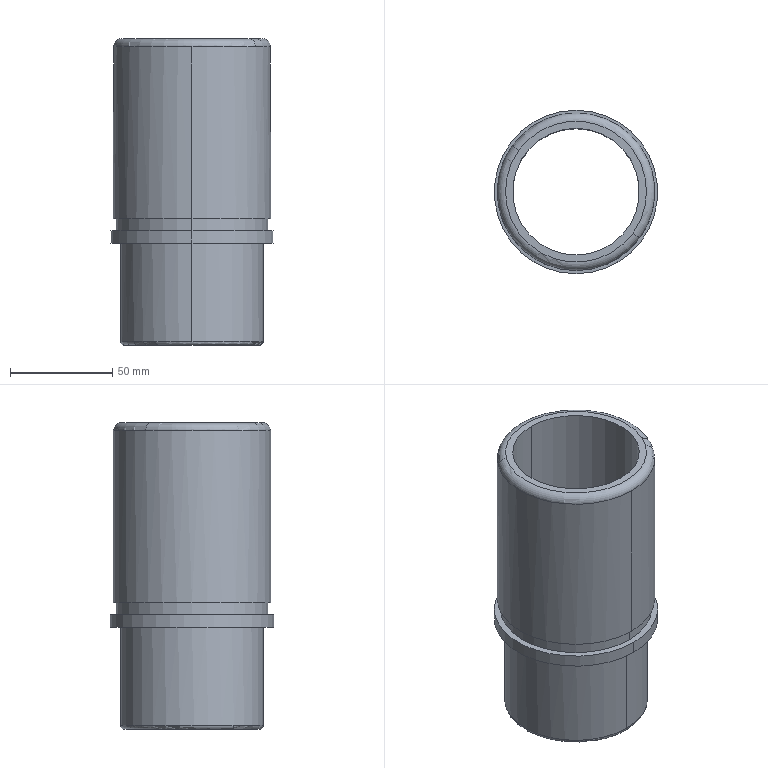Part | 1 solid | 19 faces | box 80 x 80 x 150 mm | volume 204312 mm3 | cylinder 10 | plane 5 | torus 4 | commonest cylinder face diameters 62 x2 70 x2 74.001 x2 77 x2 80 x2
STEP:
#1=CARTESIAN_POINT('',(0.,0.,0.));
#2=DIRECTION('',(0.,0.,1.));
#3=DIRECTION('',(1.,0.,0.));
#4=AXIS2_PLACEMENT_3D('',#1,#2,#3);
#5=CARTESIAN_POINT('',(-480.,16.5,-286.55));
#6=VERTEX_POINT('',#5);
#7=CARTESIAN_POINT('',(-480.,16.5,-334.55));
#8=VERTEX_POINT('',#7);
#9=CARTESIAN_POINT('',(-480.,16.5,-286.55));
#10=DIRECTION('',(0.,0.,-1.));
#11=VECTOR('',#10,1.);
#12=LINE('',#9,#11);
#13=CARTESIAN_POINT('',(-480.,-18.5,-169.951));
#14=DIRECTION('',(0.,0.,-1.));
#15=DIRECTION('',(-1.,0.,0.));
#16=AXIS2_PLACEMENT_3D('',#13,#14,#15);
#17=CYLINDRICAL_SURFACE('',#16,35.);
#18=CARTESIAN_POINT('',(1.571,116.599));
#19=DIRECTION('',(0.,1.));
#20=VECTOR('',#19,1.);
#21=LINE('',#18,#20);
#22=(GEOMETRIC_REPRESENTATION_CONTEXT(2)PARAMETRIC_REPRESENTATION_CONTEXT()REPRESENTATION_CONTEXT('',''));
#23=DEFINITIONAL_REPRESENTATION('',(#21),#22);
#24=PCURVE('',#17,#23);
#25=CARTESIAN_POINT('',(-480.,-18.5,-169.951));
#26=DIRECTION('',(0.,0.,-1.));
#27=DIRECTION('',(1.,0.,0.));
#28=AXIS2_PLACEMENT_3D('',#25,#26,#27);
#29=CYLINDRICAL_SURFACE('',#28,35.);
#30=CARTESIAN_POINT('',(4.712,116.599));
#31=DIRECTION('',(0.,1.));
#32=VECTOR('',#31,1.);
#33=LINE('',#30,#32);
#34=(GEOMETRIC_REPRESENTATION_CONTEXT(2)PARAMETRIC_REPRESENTATION_CONTEXT()REPRESENTATION_CONTEXT('',''));
#35=DEFINITIONAL_REPRESENTATION('',(#33),#34);
#36=PCURVE('',#29,#35);
#37=SURFACE_CURVE('',#12,(#24,#36),.PCURVE_S1.);
#38=EDGE_CURVE('',#6,#8,#37,.T.);
#39=ORIENTED_EDGE('',*,*,#38,.F.);
#40=CARTESIAN_POINT('',(-480.,-53.5,-286.55));
#41=VERTEX_POINT('',#40);
#42=CARTESIAN_POINT('',(-480.,-18.5,-286.55));
#43=DIRECTION('',(0.,0.,-1.));
#44=DIRECTION('',(0.,-1.,0.));
#45=AXIS2_PLACEMENT_3D('',#42,#43,#44);
#46=CIRCLE('',#45,35.);
#47=CARTESIAN_POINT('',(-1.571,116.599));
#48=DIRECTION('',(1.,0.));
#49=VECTOR('',#48,1.);
#50=LINE('',#47,#49);
#51=(GEOMETRIC_REPRESENTATION_CONTEXT(2)PARAMETRIC_REPRESENTATION_CONTEXT()REPRESENTATION_CONTEXT('',''));
#52=DEFINITIONAL_REPRESENTATION('',(#50),#51);
#53=PCURVE('',#17,#52);
#54=CARTESIAN_POINT('',(-530.585,-18.5,-286.55));
#55=DIRECTION('',(0.,0.,-1.));
#56=DIRECTION('',(0.,-1.,0.));
#57=AXIS2_PLACEMENT_3D('',#54,#55,#56);
#58=PLANE('',#57);
#59=CARTESIAN_POINT('',(0.,-50.585));
#60=DIRECTION('',(1.,0.));
#61=AXIS2_PLACEMENT_2D('',#59,#60);
#62=CIRCLE('',#61,35.);
#63=(GEOMETRIC_REPRESENTATION_CONTEXT(2)PARAMETRIC_REPRESENTATION_CONTEXT()REPRESENTATION_CONTEXT('',''));
#64=DEFINITIONAL_REPRESENTATION('',(#62),#63);
#65=PCURVE('',#58,#64);
#66=SURFACE_CURVE('',#46,(#53,#65),.PCURVE_S1.);
#67=EDGE_CURVE('',#6,#41,#66,.T.);
#68=ORIENTED_EDGE('',*,*,#67,.T.);
#69=CARTESIAN_POINT('',(-480.,-53.5,-334.55));
#70=VERTEX_POINT('',#69);
#71=CARTESIAN_POINT('',(-480.,-53.5,-286.55));
#72=DIRECTION('',(0.,0.,-1.));
#73=VECTOR('',#72,1.);
#74=LINE('',#71,#73);
#75=CARTESIAN_POINT('',(4.712,116.599));
#76=DIRECTION('',(0.,1.));
#77=VECTOR('',#76,1.);
#78=LINE('',#75,#77);
#79=(GEOMETRIC_REPRESENTATION_CONTEXT(2)PARAMETRIC_REPRESENTATION_CONTEXT()REPRESENTATION_CONTEXT('',''));
#80=DEFINITIONAL_REPRESENTATION('',(#78),#79);
#81=PCURVE('',#17,#80);
#82=CARTESIAN_POINT('',(1.571,116.599));
#83=DIRECTION('',(0.,1.));
#84=VECTOR('',#83,1.);
#85=LINE('',#82,#84);
#86=(GEOMETRIC_REPRESENTATION_CONTEXT(2)PARAMETRIC_REPRESENTATION_CONTEXT()REPRESENTATION_CONTEXT('',''));
#87=DEFINITIONAL_REPRESENTATION('',(#85),#86);
#88=PCURVE('',#29,#87);
#89=SURFACE_CURVE('',#74,(#81,#88),.PCURVE_S1.);
#90=EDGE_CURVE('',#41,#70,#89,.T.);
#91=ORIENTED_EDGE('',*,*,#90,.T.);
#92=CARTESIAN_POINT('',(-451.684,2.072,-334.55));
#93=VERTEX_POINT('',#92);
#94=CARTESIAN_POINT('',(-480.,-18.5,-334.55));
#95=DIRECTION('',(0.,0.,-1.));
#96=DIRECTION('',(0.,-1.,0.));
#97=AXIS2_PLACEMENT_3D('',#94,#95,#96);
#98=CIRCLE('',#97,35.);
#99=CARTESIAN_POINT('',(-1.571,164.599));
#100=DIRECTION('',(1.,0.));
#101=VECTOR('',#100,1.);
#102=LINE('',#99,#101);
#103=(GEOMETRIC_REPRESENTATION_CONTEXT(2)PARAMETRIC_REPRESENTATION_CONTEXT()REPRESENTATION_CONTEXT('',''));
#104=DEFINITIONAL_REPRESENTATION('',(#102),#103);
#105=PCURVE('',#17,#104);
#106=CARTESIAN_POINT('',(-480.,-18.5,-334.55));
#107=DIRECTION('',(0.,0.,-1.));
#108=DIRECTION('',(-0.5878,0.809,0.));
#109=AXIS2_PLACEMENT_3D('',#106,#107,#108);
#110=TOROIDAL_SURFACE('',#109,33.,2.);
#111=CARTESIAN_POINT('',(-2.513,0.));
#112=DIRECTION('',(1.,0.));
#113=VECTOR('',#112,1.);
#114=LINE('',#111,#113);
#115=(GEOMETRIC_REPRESENTATION_CONTEXT(2)PARAMETRIC_REPRESENTATION_CONTEXT()REPRESENTATION_CONTEXT('',''));
#116=DEFINITIONAL_REPRESENTATION('',(#114),#115);
#117=PCURVE('',#110,#116);
#118=SURFACE_CURVE('',#98,(#105,#117),.PCURVE_S1.);
#119=EDGE_CURVE('',#93,#70,#118,.T.);
#120=ORIENTED_EDGE('',*,*,#119,.F.);
#121=CARTESIAN_POINT('',(-480.,-18.5,-334.55));
#122=DIRECTION('',(0.,0.,-1.));
#123=DIRECTION('',(0.,-1.,0.));
#124=AXIS2_PLACEMENT_3D('',#121,#122,#123);
#125=CIRCLE('',#124,35.);
#126=CARTESIAN_POINT('',(-1.571,164.599));
#127=DIRECTION('',(1.,0.));
#128=VECTOR('',#127,1.);
#129=LINE('',#126,#128);
#130=(GEOMETRIC_REPRESENTATION_CONTEXT(2)PARAMETRIC_REPRESENTATION_CONTEXT()REPRESENTATION_CONTEXT('',''));
#131=DEFINITIONAL_REPRESENTATION('',(#129),#130);
#132=PCURVE('',#17,#131);
#133=CARTESIAN_POINT('',(-480.,-18.5,-334.55));
#134=DIRECTION('',(0.,0.,-1.));
#135=DIRECTION('',(0.5878,-0.809,0.));
#136=AXIS2_PLACEMENT_3D('',#133,#134,#135);
#137=TOROIDAL_SURFACE('',#136,33.,2.);
#138=CARTESIAN_POINT('',(0.6283,0.));
#139=DIRECTION('',(1.,0.));
#140=VECTOR('',#139,1.);
#141=LINE('',#138,#140);
#142=(GEOMETRIC_REPRESENTATION_CONTEXT(2)PARAMETRIC_REPRESENTATION_CONTEXT()REPRESENTATION_CONTEXT('',''));
#143=DEFINITIONAL_REPRESENTATION('',(#141),#142);
#144=PCURVE('',#137,#143);
#145=SURFACE_CURVE('',#125,(#132,#144),.PCURVE_S1.);
#146=EDGE_CURVE('',#8,#93,#145,.T.);
#147=ORIENTED_EDGE('',*,*,#146,.F.);
#148=EDGE_LOOP('',(#39,#68,#91,#120,#147));
#149=FACE_BOUND('',#148,.T.);
#150=ADVANCED_FACE('',(#149),#17,.T.);
#151=CARTESIAN_POINT('',(-480.,-58.5,-286.55));
#152=VERTEX_POINT('',#151);
#153=CARTESIAN_POINT('',(-480.,21.5,-286.55));
#154=VERTEX_POINT('',#153);
#155=CARTESIAN_POINT('',(-480.,-18.5,-286.55));
#156=DIRECTION('',(0.,0.,-1.));
#157=DIRECTION('',(0.,-1.,0.));
#158=AXIS2_PLACEMENT_3D('',#155,#156,#157);
#159=CIRCLE('',#158,40.);
#160=CARTESIAN_POINT('',(0.,-50.585));
#161=DIRECTION('',(1.,0.));
#162=AXIS2_PLACEMENT_2D('',#160,#161);
#163=CIRCLE('',#162,40.);
#164=(GEOMETRIC_REPRESENTATION_CONTEXT(2)PARAMETRIC_REPRESENTATION_CONTEXT()REPRESENTATION_CONTEXT('',''));
#165=DEFINITIONAL_REPRESENTATION('',(#163),#164);
#166=PCURVE('',#58,#165);
#167=CARTESIAN_POINT('',(-480.,-18.5,-169.951));
#168=DIRECTION('',(0.,0.,-1.));
#169=DIRECTION('',(1.,0.,0.));
#170=AXIS2_PLACEMENT_3D('',#167,#168,#169);
#171=CYLINDRICAL_SURFACE('',#170,40.);
#172=CARTESIAN_POINT('',(1.571,116.599));
#173=DIRECTION('',(1.,0.));
#174=VECTOR('',#173,1.);
#175=LINE('',#172,#174);
#176=(GEOMETRIC_REPRESENTATION_CONTEXT(2)PARAMETRIC_REPRESENTATION_CONTEXT()REPRESENTATION_CONTEXT('',''));
#177=DEFINITIONAL_REPRESENTATION('',(#175),#176);
#178=PCURVE('',#171,#177);
#179=SURFACE_CURVE('',#159,(#166,#178),.PCURVE_S1.);
#180=EDGE_CURVE('',#152,#154,#179,.T.);
#181=ORIENTED_EDGE('',*,*,#180,.T.);
#182=CARTESIAN_POINT('',(-480.,-18.5,-286.55));
#183=DIRECTION('',(0.,0.,-1.));
#184=DIRECTION('',(0.,-1.,0.));
#185=AXIS2_PLACEMENT_3D('',#182,#183,#184);
#186=CIRCLE('',#185,40.);
#187=CARTESIAN_POINT('',(0.,-50.585));
#188=DIRECTION('',(1.,0.));
#189=AXIS2_PLACEMENT_2D('',#187,#188);
#190=CIRCLE('',#189,40.);
#191=(GEOMETRIC_REPRESENTATION_CONTEXT(2)PARAMETRIC_REPRESENTATION_CONTEXT()REPRESENTATION_CONTEXT('',''));
#192=DEFINITIONAL_REPRESENTATION('',(#190),#191);
#193=PCURVE('',#58,#192);
#194=CARTESIAN_POINT('',(-480.,-18.5,-169.951));
#195=DIRECTION('',(0.,0.,-1.));
#196=DIRECTION('',(-1.,0.,0.));
#197=AXIS2_PLACEMENT_3D('',#194,#195,#196);
#198=CYLINDRICAL_SURFACE('',#197,40.);
#199=CARTESIAN_POINT('',(-1.571,116.599));
#200=DIRECTION('',(1.,0.));
#201=VECTOR('',#200,1.);
#202=LINE('',#199,#201);
#203=(GEOMETRIC_REPRESENTATION_CONTEXT(2)PARAMETRIC_REPRESENTATION_CONTEXT()REPRESENTATION_CONTEXT('',''));
#204=DEFINITIONAL_REPRESENTATION('',(#202),#203);
#205=PCURVE('',#198,#204);
#206=SURFACE_CURVE('',#186,(#193,#205),.PCURVE_S1.);
#207=EDGE_CURVE('',#154,#152,#206,.T.);
#208=ORIENTED_EDGE('',*,*,#207,.T.);
#209=EDGE_LOOP('',(#181,#208));
#210=FACE_BOUND('',#209,.T.);
#211=ORIENTED_EDGE('',*,*,#67,.F.);
#212=CARTESIAN_POINT('',(-480.,-18.5,-286.55));
#213=DIRECTION('',(0.,0.,-1.));
#214=DIRECTION('',(0.,-1.,0.));
#215=AXIS2_PLACEMENT_3D('',#212,#213,#214);
#216=CIRCLE('',#215,35.);
#217=CARTESIAN_POINT('',(0.,-50.585));
#218=DIRECTION('',(1.,0.));
#219=AXIS2_PLACEMENT_2D('',#217,#218);
#220=CIRCLE('',#219,35.);
#221=(GEOMETRIC_REPRESENTATION_CONTEXT(2)PARAMETRIC_REPRESENTATION_CONTEXT()REPRESENTATION_CONTEXT('',''));
#222=DEFINITIONAL_REPRESENTATION('',(#220),#221);
#223=PCURVE('',#58,#222);
#224=CARTESIAN_POINT('',(1.571,116.599));
#225=DIRECTION('',(1.,0.));
#226=VECTOR('',#225,1.);
#227=LINE('',#224,#226);
#228=(GEOMETRIC_REPRESENTATION_CONTEXT(2)PARAMETRIC_REPRESENTATION_CONTEXT()REPRESENTATION_CONTEXT('',''));
#229=DEFINITIONAL_REPRESENTATION('',(#227),#228);
#230=PCURVE('',#29,#229);
#231=SURFACE_CURVE('',#216,(#223,#230),.PCURVE_S1.);
#232=EDGE_CURVE('',#41,#6,#231,.T.);
#233=ORIENTED_EDGE('',*,*,#232,.F.);
#234=EDGE_LOOP('',(#211,#233));
#235=FACE_BOUND('',#234,.T.);
#236=ADVANCED_FACE('',(#210,#235),#58,.T.);
#237=CARTESIAN_POINT('',(-480.,21.5,-280.55));
#238=VERTEX_POINT('',#237);
#239=CARTESIAN_POINT('',(-480.,21.5,-280.55));
#240=DIRECTION('',(0.,0.,-1.));
#241=VECTOR('',#240,1.);
#242=LINE('',#239,#241);
#243=CARTESIAN_POINT('',(1.571,110.599));
#244=DIRECTION('',(0.,1.));
#245=VECTOR('',#244,1.);
#246=LINE('',#243,#245);
#247=(GEOMETRIC_REPRESENTATION_CONTEXT(2)PARAMETRIC_REPRESENTATION_CONTEXT()REPRESENTATION_CONTEXT('',''));
#248=DEFINITIONAL_REPRESENTATION('',(#246),#247);
#249=PCURVE('',#198,#248);
#250=CARTESIAN_POINT('',(4.712,110.599));
#251=DIRECTION('',(0.,1.));
#252=VECTOR('',#251,1.);
#253=LINE('',#250,#252);
#254=(GEOMETRIC_REPRESENTATION_CONTEXT(2)PARAMETRIC_REPRESENTATION_CONTEXT()REPRESENTATION_CONTEXT('',''));
#255=DEFINITIONAL_REPRESENTATION('',(#253),#254);
#256=PCURVE('',#171,#255);
#257=SURFACE_CURVE('',#242,(#249,#256),.PCURVE_S1.);
#258=EDGE_CURVE('',#238,#154,#257,.T.);
#259=ORIENTED_EDGE('',*,*,#258,.F.);
#260=CARTESIAN_POINT('',(-480.,-58.5,-280.55));
#261=VERTEX_POINT('',#260);
#262=CARTESIAN_POINT('',(-480.,-18.5,-280.55));
#263=DIRECTION('',(0.,0.,-1.));
#264=DIRECTION('',(0.,-1.,0.));
#265=AXIS2_PLACEMENT_3D('',#262,#263,#264);
#266=CIRCLE('',#265,40.);
#267=CARTESIAN_POINT('',(-1.571,110.599));
#268=DIRECTION('',(1.,0.));
#269=VECTOR('',#268,1.);
#270=LINE('',#267,#269);
#271=(GEOMETRIC_REPRESENTATION_CONTEXT(2)PARAMETRIC_REPRESENTATION_CONTEXT()REPRESENTATION_CONTEXT('',''));
#272=DEFINITIONAL_REPRESENTATION('',(#270),#271);
#273=PCURVE('',#198,#272);
#274=CARTESIAN_POINT('',(-539.585,-18.5,-280.55));
#275=DIRECTION('',(0.,0.,1.));
#276=DIRECTION('',(0.,1.,0.));
#277=AXIS2_PLACEMENT_3D('',#274,#275,#276);
#278=PLANE('',#277);
#279=CARTESIAN_POINT('',(-40.,-59.585));
#280=CARTESIAN_POINT('',(-40.,9.697));
#281=CARTESIAN_POINT('',(20.,-24.944));
#282=CARTESIAN_POINT('',(80.,-59.585));
#283=CARTESIAN_POINT('',(20.,-94.226));
#284=CARTESIAN_POINT('',(-40.,-128.867));
#285=CARTESIAN_POINT('',(-40.,-59.585));
#286=(BOUNDED_CURVE()B_SPLINE_CURVE(2,(#279,#280,#281,#282,#283,#284,#285),.UNSPECIFIED.,.T.,.F.)B_SPLINE_CURVE_WITH_KNOTS((1,2,2,2,2,1),(-2.094,0.,2.094,4.189,6.283,8.378),.UNSPECIFIED.)CURVE()GEOMETRIC_REPRESENTATION_ITEM()RATIONAL_B_SPLINE_CURVE((1.,0.5,1.,0.5,1.,0.5,1.))REPRESENTATION_ITEM(''));
#287=(GEOMETRIC_REPRESENTATION_CONTEXT(2)PARAMETRIC_REPRESENTATION_CONTEXT()REPRESENTATION_CONTEXT('',''));
#288=DEFINITIONAL_REPRESENTATION('',(#286),#287);
#289=PCURVE('',#278,#288);
#290=SURFACE_CURVE('',#266,(#273,#289),.PCURVE_S1.);
#291=EDGE_CURVE('',#238,#261,#290,.T.);
#292=ORIENTED_EDGE('',*,*,#291,.T.);
#293=CARTESIAN_POINT('',(-480.,-58.5,-280.55));
#294=DIRECTION('',(0.,0.,-1.));
#295=VECTOR('',#294,1.);
#296=LINE('',#293,#295);
#297=CARTESIAN_POINT('',(4.712,110.599));
#298=DIRECTION('',(0.,1.));
#299=VECTOR('',#298,1.);
#300=LINE('',#297,#299);
#301=(GEOMETRIC_REPRESENTATION_CONTEXT(2)PARAMETRIC_REPRESENTATION_CONTEXT()REPRESENTATION_CONTEXT('',''));
#302=DEFINITIONAL_REPRESENTATION('',(#300),#301);
#303=PCURVE('',#198,#302);
#304=CARTESIAN_POINT('',(1.571,110.599));
#305=DIRECTION('',(0.,1.));
#306=VECTOR('',#305,1.);
#307=LINE('',#304,#306);
#308=(GEOMETRIC_REPRESENTATION_CONTEXT(2)PARAMETRIC_REPRESENTATION_CONTEXT()REPRESENTATION_CONTEXT('',''));
#309=DEFINITIONAL_REPRESENTATION('',(#307),#308);
#310=PCURVE('',#171,#309);
#311=SURFACE_CURVE('',#296,(#303,#310),.PCURVE_S1.);
#312=EDGE_CURVE('',#261,#152,#311,.T.);
#313=ORIENTED_EDGE('',*,*,#312,.T.);
#314=ORIENTED_EDGE('',*,*,#207,.F.);
#315=EDGE_LOOP('',(#259,#292,#313,#314));
#316=FACE_BOUND('',#315,.T.);
#317=ADVANCED_FACE('',(#316),#198,.T.);
#318=ORIENTED_EDGE('',*,*,#291,.F.);
#319=CARTESIAN_POINT('',(-480.,-18.5,-280.55));
#320=DIRECTION('',(0.,0.,-1.));
#321=DIRECTION('',(0.,-1.,0.));
#322=AXIS2_PLACEMENT_3D('',#319,#320,#321);
#323=CIRCLE('',#322,40.);
#324=CARTESIAN_POINT('',(-40.,-59.585));
#325=CARTESIAN_POINT('',(-40.,9.697));
#326=CARTESIAN_POINT('',(20.,-24.944));
#327=CARTESIAN_POINT('',(80.,-59.585));
#328=CARTESIAN_POINT('',(20.,-94.226));
#329=CARTESIAN_POINT('',(-40.,-128.867));
#330=CARTESIAN_POINT('',(-40.,-59.585));
#331=(BOUNDED_CURVE()B_SPLINE_CURVE(2,(#324,#325,#326,#327,#328,#329,#330),.UNSPECIFIED.,.T.,.F.)B_SPLINE_CURVE_WITH_KNOTS((1,2,2,2,2,1),(-2.094,0.,2.094,4.189,6.283,8.378),.UNSPECIFIED.)CURVE()GEOMETRIC_REPRESENTATION_ITEM()RATIONAL_B_SPLINE_CURVE((1.,0.5,1.,0.5,1.,0.5,1.))REPRESENTATION_ITEM(''));
#332=(GEOMETRIC_REPRESENTATION_CONTEXT(2)PARAMETRIC_REPRESENTATION_CONTEXT()REPRESENTATION_CONTEXT('',''));
#333=DEFINITIONAL_REPRESENTATION('',(#331),#332);
#334=PCURVE('',#278,#333);
#335=CARTESIAN_POINT('',(1.571,110.599));
#336=DIRECTION('',(1.,0.));
#337=VECTOR('',#336,1.);
#338=LINE('',#335,#337);
#339=(GEOMETRIC_REPRESENTATION_CONTEXT(2)PARAMETRIC_REPRESENTATION_CONTEXT()REPRESENTATION_CONTEXT('',''));
#340=DEFINITIONAL_REPRESENTATION('',(#338),#339);
#341=PCURVE('',#171,#340);
#342=SURFACE_CURVE('',#323,(#334,#341),.PCURVE_S1.);
#343=EDGE_CURVE('',#261,#238,#342,.T.);
#344=ORIENTED_EDGE('',*,*,#343,.F.);
#345=EDGE_LOOP('',(#318,#344));
#346=FACE_BOUND('',#345,.T.);
#347=CARTESIAN_POINT('',(-480.,-55.5,-280.55));
#348=VERTEX_POINT('',#347);
#349=CARTESIAN_POINT('',(-480.,18.5,-280.55));
#350=VERTEX_POINT('',#349);
#351=CARTESIAN_POINT('',(-480.,-18.5,-280.55));
#352=DIRECTION('',(0.,0.,-1.));
#353=DIRECTION('',(0.,-1.,0.));
#354=AXIS2_PLACEMENT_3D('',#351,#352,#353);
#355=CIRCLE('',#354,37.);
#356=CARTESIAN_POINT('',(-37.,-59.585));
#357=CARTESIAN_POINT('',(-37.,4.501));
#358=CARTESIAN_POINT('',(18.5,-27.542));
#359=CARTESIAN_POINT('',(74.001,-59.585));
#360=CARTESIAN_POINT('',(18.5,-91.628));
#361=CARTESIAN_POINT('',(-37.,-123.672));
#362=CARTESIAN_POINT('',(-37.,-59.585));
#363=(BOUNDED_CURVE()B_SPLINE_CURVE(2,(#356,#357,#358,#359,#360,#361,#362),.UNSPECIFIED.,.T.,.F.)B_SPLINE_CURVE_WITH_KNOTS((1,2,2,2,2,1),(-2.094,0.,2.094,4.189,6.283,8.378),.UNSPECIFIED.)CURVE()GEOMETRIC_REPRESENTATION_ITEM()RATIONAL_B_SPLINE_CURVE((1.,0.5,1.,0.5,1.,0.5,1.))REPRESENTATION_ITEM(''));
#364=(GEOMETRIC_REPRESENTATION_CONTEXT(2)PARAMETRIC_REPRESENTATION_CONTEXT()REPRESENTATION_CONTEXT('',''));
#365=DEFINITIONAL_REPRESENTATION('',(#363),#364);
#366=PCURVE('',#278,#365);
#367=CARTESIAN_POINT('',(-480.,-18.5,-169.951));
#368=DIRECTION('',(0.,0.,-1.));
#369=DIRECTION('',(1.,0.,0.));
#370=AXIS2_PLACEMENT_3D('',#367,#368,#369);
#371=CYLINDRICAL_SURFACE('',#370,37.);
#372=CARTESIAN_POINT('',(1.571,110.599));
#373=DIRECTION('',(1.,0.));
#374=VECTOR('',#373,1.);
#375=LINE('',#372,#374);
#376=(GEOMETRIC_REPRESENTATION_CONTEXT(2)PARAMETRIC_REPRESENTATION_CONTEXT()REPRESENTATION_CONTEXT('',''));
#377=DEFINITIONAL_REPRESENTATION('',(#375),#376);
#378=PCURVE('',#371,#377);
#379=SURFACE_CURVE('',#355,(#366,#378),.PCURVE_S1.);
#380=EDGE_CURVE('',#348,#350,#379,.T.);
#381=ORIENTED_EDGE('',*,*,#380,.T.);
#382=CARTESIAN_POINT('',(-480.,-18.5,-280.55));
#383=DIRECTION('',(0.,0.,-1.));
#384=DIRECTION('',(0.,-1.,0.));
#385=AXIS2_PLACEMENT_3D('',#382,#383,#384);
#386=CIRCLE('',#385,37.);
#387=CARTESIAN_POINT('',(-37.,-59.585));
#388=CARTESIAN_POINT('',(-37.,4.501));
#389=CARTESIAN_POINT('',(18.5,-27.542));
#390=CARTESIAN_POINT('',(74.001,-59.585));
#391=CARTESIAN_POINT('',(18.5,-91.628));
#392=CARTESIAN_POINT('',(-37.,-123.672));
#393=CARTESIAN_POINT('',(-37.,-59.585));
#394=(BOUNDED_CURVE()B_SPLINE_CURVE(2,(#387,#388,#389,#390,#391,#392,#393),.UNSPECIFIED.,.T.,.F.)B_SPLINE_CURVE_WITH_KNOTS((1,2,2,2,2,1),(-2.094,0.,2.094,4.189,6.283,8.378),.UNSPECIFIED.)CURVE()GEOMETRIC_REPRESENTATION_ITEM()RATIONAL_B_SPLINE_CURVE((1.,0.5,1.,0.5,1.,0.5,1.))REPRESENTATION_ITEM(''));
#395=(GEOMETRIC_REPRESENTATION_CONTEXT(2)PARAMETRIC_REPRESENTATION_CONTEXT()REPRESENTATION_CONTEXT('',''));
#396=DEFINITIONAL_REPRESENTATION('',(#394),#395);
#397=PCURVE('',#278,#396);
#398=CARTESIAN_POINT('',(-480.,-18.5,-169.951));
#399=DIRECTION('',(0.,0.,-1.));
#400=DIRECTION('',(-1.,0.,0.));
#401=AXIS2_PLACEMENT_3D('',#398,#399,#400);
#402=CYLINDRICAL_SURFACE('',#401,37.);
#403=CARTESIAN_POINT('',(-1.571,110.599));
#404=DIRECTION('',(1.,0.));
#405=VECTOR('',#404,1.);
#406=LINE('',#403,#405);
#407=(GEOMETRIC_REPRESENTATION_CONTEXT(2)PARAMETRIC_REPRESENTATION_CONTEXT()REPRESENTATION_CONTEXT('',''));
#408=DEFINITIONAL_REPRESENTATION('',(#406),#407);
#409=PCURVE('',#402,#408);
#410=SURFACE_CURVE('',#386,(#397,#409),.PCURVE_S1.);
#411=EDGE_CURVE('',#350,#348,#410,.T.);
#412=ORIENTED_EDGE('',*,*,#411,.T.);
#413=EDGE_LOOP('',(#381,#412));
#414=FACE_BOUND('',#413,.T.);
#415=ADVANCED_FACE('',(#346,#414),#278,.T.);
#416=CARTESIAN_POINT('',(-480.,18.5,-274.55));
#417=VERTEX_POINT('',#416);
#418=CARTESIAN_POINT('',(-480.,18.5,-274.55));
#419=DIRECTION('',(0.,0.,-1.));
#420=VECTOR('',#419,1.);
#421=LINE('',#418,#420);
#422=CARTESIAN_POINT('',(1.571,104.599));
#423=DIRECTION('',(0.,1.));
#424=VECTOR('',#423,1.);
#425=LINE('',#422,#424);
#426=(GEOMETRIC_REPRESENTATION_CONTEXT(2)PARAMETRIC_REPRESENTATION_CONTEXT()REPRESENTATION_CONTEXT('',''));
#427=DEFINITIONAL_REPRESENTATION('',(#425),#426);
#428=PCURVE('',#402,#427);
#429=CARTESIAN_POINT('',(4.712,104.599));
#430=DIRECTION('',(0.,1.));
#431=VECTOR('',#430,1.);
#432=LINE('',#429,#431);
#433=(GEOMETRIC_REPRESENTATION_CONTEXT(2)PARAMETRIC_REPRESENTATION_CONTEXT()REPRESENTATION_CONTEXT('',''));
#434=DEFINITIONAL_REPRESENTATION('',(#432),#433);
#435=PCURVE('',#371,#434);
#436=SURFACE_CURVE('',#421,(#428,#435),.PCURVE_S1.);
#437=EDGE_CURVE('',#417,#350,#436,.T.);
#438=ORIENTED_EDGE('',*,*,#437,.F.);
#439=CARTESIAN_POINT('',(-480.,-55.5,-274.55));
#440=VERTEX_POINT('',#439);
#441=CARTESIAN_POINT('',(-480.,-18.5,-274.55));
#442=DIRECTION('',(0.,0.,1.));
#443=DIRECTION('',(0.,-1.,0.));
#444=AXIS2_PLACEMENT_3D('',#441,#442,#443);
#445=CIRCLE('',#444,37.);
#446=CARTESIAN_POINT('',(4.712,104.599));
#447=DIRECTION('',(-1.,0.));
#448=VECTOR('',#447,1.);
#449=LINE('',#446,#448);
#450=(GEOMETRIC_REPRESENTATION_CONTEXT(2)PARAMETRIC_REPRESENTATION_CONTEXT()REPRESENTATION_CONTEXT('',''));
#451=DEFINITIONAL_REPRESENTATION('',(#449),#450);
#452=PCURVE('',#402,#451);
#453=CARTESIAN_POINT('',(-539.585,-18.5,-274.55));
#454=DIRECTION('',(0.,0.,1.));
#455=DIRECTION('',(0.,1.,0.));
#456=AXIS2_PLACEMENT_3D('',#453,#454,#455);
#457=PLANE('',#456);
#458=CARTESIAN_POINT('',(0.,-59.585));
#459=DIRECTION('',(-1.,0.));
#460=AXIS2_PLACEMENT_2D('',#458,#459);
#461=CIRCLE('',#460,37.);
#462=(GEOMETRIC_REPRESENTATION_CONTEXT(2)PARAMETRIC_REPRESENTATION_CONTEXT()REPRESENTATION_CONTEXT('',''));
#463=DEFINITIONAL_REPRESENTATION('',(#461),#462);
#464=PCURVE('',#457,#463);
#465=SURFACE_CURVE('',#445,(#452,#464),.PCURVE_S1.);
#466=EDGE_CURVE('',#440,#417,#465,.T.);
#467=ORIENTED_EDGE('',*,*,#466,.F.);
#468=CARTESIAN_POINT('',(-480.,-55.5,-274.55));
#469=DIRECTION('',(0.,0.,-1.));
#470=VECTOR('',#469,1.);
#471=LINE('',#468,#470);
#472=CARTESIAN_POINT('',(4.712,104.599));
#473=DIRECTION('',(0.,1.));
#474=VECTOR('',#473,1.);
#475=LINE('',#472,#474);
#476=(GEOMETRIC_REPRESENTATION_CONTEXT(2)PARAMETRIC_REPRESENTATION_CONTEXT()REPRESENTATION_CONTEXT('',''));
#477=DEFINITIONAL_REPRESENTATION('',(#475),#476);
#478=PCURVE('',#402,#477);
#479=CARTESIAN_POINT('',(1.571,104.599));
#480=DIRECTION('',(0.,1.));
#481=VECTOR('',#480,1.);
#482=LINE('',#479,#481);
#483=(GEOMETRIC_REPRESENTATION_CONTEXT(2)PARAMETRIC_REPRESENTATION_CONTEXT()REPRESENTATION_CONTEXT('',''));
#484=DEFINITIONAL_REPRESENTATION('',(#482),#483);
#485=PCURVE('',#371,#484);
#486=SURFACE_CURVE('',#471,(#478,#485),.PCURVE_S1.);
#487=EDGE_CURVE('',#440,#348,#486,.T.);
#488=ORIENTED_EDGE('',*,*,#487,.T.);
#489=ORIENTED_EDGE('',*,*,#411,.F.);
#490=EDGE_LOOP('',(#438,#467,#488,#489));
#491=FACE_BOUND('',#490,.T.);
#492=ADVANCED_FACE('',(#491),#402,.T.);
#493=ORIENTED_EDGE('',*,*,#466,.T.);
#494=CARTESIAN_POINT('',(-480.,-18.5,-274.55));
#495=DIRECTION('',(0.,0.,1.));
#496=DIRECTION('',(0.,-1.,0.));
#497=AXIS2_PLACEMENT_3D('',#494,#495,#496);
#498=CIRCLE('',#497,37.);
#499=CARTESIAN_POINT('',(0.,-59.585));
#500=DIRECTION('',(-1.,0.));
#501=AXIS2_PLACEMENT_2D('',#499,#500);
#502=CIRCLE('',#501,37.);
#503=(GEOMETRIC_REPRESENTATION_CONTEXT(2)PARAMETRIC_REPRESENTATION_CONTEXT()REPRESENTATION_CONTEXT('',''));
#504=DEFINITIONAL_REPRESENTATION('',(#502),#503);
#505=PCURVE('',#457,#504);
#506=CARTESIAN_POINT('',(7.854,104.599));
#507=DIRECTION('',(-1.,0.));
#508=VECTOR('',#507,1.);
#509=LINE('',#506,#508);
#510=(GEOMETRIC_REPRESENTATION_CONTEXT(2)PARAMETRIC_REPRESENTATION_CONTEXT()REPRESENTATION_CONTEXT('',''));
#511=DEFINITIONAL_REPRESENTATION('',(#509),#510);
#512=PCURVE('',#371,#511);
#513=SURFACE_CURVE('',#498,(#505,#512),.PCURVE_S1.);
#514=EDGE_CURVE('',#417,#440,#513,.T.);
#515=ORIENTED_EDGE('',*,*,#514,.T.);
#516=EDGE_LOOP('',(#493,#515));
#517=FACE_BOUND('',#516,.T.);
#518=CARTESIAN_POINT('',(-480.,-57.,-274.55));
#519=VERTEX_POINT('',#518);
#520=CARTESIAN_POINT('',(-480.,20.,-274.55));
#521=VERTEX_POINT('',#520);
#522=CARTESIAN_POINT('',(-480.,-18.5,-274.55));
#523=DIRECTION('',(0.,0.,-1.));
#524=DIRECTION('',(0.,-1.,0.));
#525=AXIS2_PLACEMENT_3D('',#522,#523,#524);
#526=CIRCLE('',#525,38.5);
#527=CARTESIAN_POINT('',(-38.5,-59.585));
#528=CARTESIAN_POINT('',(-38.5,7.099));
#529=CARTESIAN_POINT('',(19.25,-26.243));
#530=CARTESIAN_POINT('',(77.,-59.585));
#531=CARTESIAN_POINT('',(19.25,-92.927));
#532=CARTESIAN_POINT('',(-38.5,-126.269));
#533=CARTESIAN_POINT('',(-38.5,-59.585));
#534=(BOUNDED_CURVE()B_SPLINE_CURVE(2,(#527,#528,#529,#530,#531,#532,#533),.UNSPECIFIED.,.T.,.F.)B_SPLINE_CURVE_WITH_KNOTS((1,2,2,2,2,1),(-2.094,0.,2.094,4.189,6.283,8.378),.UNSPECIFIED.)CURVE()GEOMETRIC_REPRESENTATION_ITEM()RATIONAL_B_SPLINE_CURVE((1.,0.5,1.,0.5,1.,0.5,1.))REPRESENTATION_ITEM(''));
#535=(GEOMETRIC_REPRESENTATION_CONTEXT(2)PARAMETRIC_REPRESENTATION_CONTEXT()REPRESENTATION_CONTEXT('',''));
#536=DEFINITIONAL_REPRESENTATION('',(#534),#535);
#537=PCURVE('',#457,#536);
#538=CARTESIAN_POINT('',(-480.,-18.5,-169.951));
#539=DIRECTION('',(0.,0.,-1.));
#540=DIRECTION('',(1.,0.,0.));
#541=AXIS2_PLACEMENT_3D('',#538,#539,#540);
#542=CYLINDRICAL_SURFACE('',#541,38.5);
#543=CARTESIAN_POINT('',(1.571,104.599));
#544=DIRECTION('',(1.,0.));
#545=VECTOR('',#544,1.);
#546=LINE('',#543,#545);
#547=(GEOMETRIC_REPRESENTATION_CONTEXT(2)PARAMETRIC_REPRESENTATION_CONTEXT()REPRESENTATION_CONTEXT('',''));
#548=DEFINITIONAL_REPRESENTATION('',(#546),#547);
#549=PCURVE('',#542,#548);
#550=SURFACE_CURVE('',#526,(#537,#549),.PCURVE_S1.);
#551=EDGE_CURVE('',#519,#521,#550,.T.);
#552=ORIENTED_EDGE('',*,*,#551,.T.);
#553=CARTESIAN_POINT('',(-480.,-18.5,-274.55));
#554=DIRECTION('',(0.,0.,-1.));
#555=DIRECTION('',(0.,-1.,0.));
#556=AXIS2_PLACEMENT_3D('',#553,#554,#555);
#557=CIRCLE('',#556,38.5);
#558=CARTESIAN_POINT('',(-38.5,-59.585));
#559=CARTESIAN_POINT('',(-38.5,7.099));
#560=CARTESIAN_POINT('',(19.25,-26.243));
#561=CARTESIAN_POINT('',(77.,-59.585));
#562=CARTESIAN_POINT('',(19.25,-92.927));
#563=CARTESIAN_POINT('',(-38.5,-126.269));
#564=CARTESIAN_POINT('',(-38.5,-59.585));
#565=(BOUNDED_CURVE()B_SPLINE_CURVE(2,(#558,#559,#560,#561,#562,#563,#564),.UNSPECIFIED.,.T.,.F.)B_SPLINE_CURVE_WITH_KNOTS((1,2,2,2,2,1),(-2.094,0.,2.094,4.189,6.283,8.378),.UNSPECIFIED.)CURVE()GEOMETRIC_REPRESENTATION_ITEM()RATIONAL_B_SPLINE_CURVE((1.,0.5,1.,0.5,1.,0.5,1.))REPRESENTATION_ITEM(''));
#566=(GEOMETRIC_REPRESENTATION_CONTEXT(2)PARAMETRIC_REPRESENTATION_CONTEXT()REPRESENTATION_CONTEXT('',''));
#567=DEFINITIONAL_REPRESENTATION('',(#565),#566);
#568=PCURVE('',#457,#567);
#569=CARTESIAN_POINT('',(-480.,-18.5,-169.951));
#570=DIRECTION('',(0.,0.,-1.));
#571=DIRECTION('',(-1.,0.,0.));
#572=AXIS2_PLACEMENT_3D('',#569,#570,#571);
#573=CYLINDRICAL_SURFACE('',#572,38.5);
#574=CARTESIAN_POINT('',(-1.571,104.599));
#575=DIRECTION('',(1.,0.));
#576=VECTOR('',#575,1.);
#577=LINE('',#574,#576);
#578=(GEOMETRIC_REPRESENTATION_CONTEXT(2)PARAMETRIC_REPRESENTATION_CONTEXT()REPRESENTATION_CONTEXT('',''));
#579=DEFINITIONAL_REPRESENTATION('',(#577),#578);
#580=PCURVE('',#573,#579);
#581=SURFACE_CURVE('',#557,(#568,#580),.PCURVE_S1.);
#582=EDGE_CURVE('',#521,#519,#581,.T.);
#583=ORIENTED_EDGE('',*,*,#582,.T.);
#584=EDGE_LOOP('',(#552,#583));
#585=FACE_BOUND('',#584,.T.);
#586=ADVANCED_FACE('',(#517,#585),#457,.F.);
#587=CARTESIAN_POINT('',(-480.,20.,-190.55));
#588=VERTEX_POINT('',#587);
#589=CARTESIAN_POINT('',(-480.,20.,-190.55));
#590=DIRECTION('',(0.,0.,-1.));
#591=VECTOR('',#590,1.);
#592=LINE('',#589,#591);
#593=CARTESIAN_POINT('',(1.571,20.599));
#594=DIRECTION('',(0.,1.));
#595=VECTOR('',#594,1.);
#596=LINE('',#593,#595);
#597=(GEOMETRIC_REPRESENTATION_CONTEXT(2)PARAMETRIC_REPRESENTATION_CONTEXT()REPRESENTATION_CONTEXT('',''));
#598=DEFINITIONAL_REPRESENTATION('',(#596),#597);
#599=PCURVE('',#573,#598);
#600=CARTESIAN_POINT('',(4.712,20.599));
#601=DIRECTION('',(0.,1.));
#602=VECTOR('',#601,1.);
#603=LINE('',#600,#602);
#604=(GEOMETRIC_REPRESENTATION_CONTEXT(2)PARAMETRIC_REPRESENTATION_CONTEXT()REPRESENTATION_CONTEXT('',''));
#605=DEFINITIONAL_REPRESENTATION('',(#603),#604);
#606=PCURVE('',#542,#605);
#607=SURFACE_CURVE('',#592,(#599,#606),.PCURVE_S1.);
#608=EDGE_CURVE('',#588,#521,#607,.T.);
#609=ORIENTED_EDGE('',*,*,#608,.F.);
#610=CARTESIAN_POINT('',(-448.853,4.13,-190.55));
#611=VERTEX_POINT('',#610);
#612=CARTESIAN_POINT('',(-480.,-18.5,-190.55));
#613=DIRECTION('',(0.,0.,-1.));
#614=DIRECTION('',(0.809,0.5878,0.));
#615=AXIS2_PLACEMENT_3D('',#612,#613,#614);
#616=CIRCLE('',#615,38.5);
#617=CARTESIAN_POINT('',(-3.77,20.599));
#618=DIRECTION('',(1.,0.));
#619=VECTOR('',#618,1.);
#620=LINE('',#617,#619);
#621=(GEOMETRIC_REPRESENTATION_CONTEXT(2)PARAMETRIC_REPRESENTATION_CONTEXT()REPRESENTATION_CONTEXT('',''));
#622=DEFINITIONAL_REPRESENTATION('',(#620),#621);
#623=PCURVE('',#573,#622);
#624=CARTESIAN_POINT('',(-480.,-18.5,-190.55));
#625=DIRECTION('',(0.,0.,1.));
#626=DIRECTION('',(-0.5878,-0.809,0.));
#627=AXIS2_PLACEMENT_3D('',#624,#625,#626);
#628=TOROIDAL_SURFACE('',#627,34.5,4.);
#629=CARTESIAN_POINT('',(9.111,0.));
#630=DIRECTION('',(-1.,0.));
#631=VECTOR('',#630,1.);
#632=LINE('',#629,#631);
#633=(GEOMETRIC_REPRESENTATION_CONTEXT(2)PARAMETRIC_REPRESENTATION_CONTEXT()REPRESENTATION_CONTEXT('',''));
#634=DEFINITIONAL_REPRESENTATION('',(#632),#633);
#635=PCURVE('',#628,#634);
#636=SURFACE_CURVE('',#616,(#623,#635),.PCURVE_S1.);
#637=EDGE_CURVE('',#588,#611,#636,.T.);
#638=ORIENTED_EDGE('',*,*,#637,.T.);
#639=CARTESIAN_POINT('',(-448.853,-41.13,-190.55));
#640=VERTEX_POINT('',#639);
#641=CARTESIAN_POINT('',(-480.,-18.5,-190.55));
#642=DIRECTION('',(0.,0.,-1.));
#643=DIRECTION('',(0.809,0.5878,0.));
#644=AXIS2_PLACEMENT_3D('',#641,#642,#643);
#645=CIRCLE('',#644,38.5);
#646=CARTESIAN_POINT('',(2.513,20.599));
#647=DIRECTION('',(1.,0.));
#648=VECTOR('',#647,1.);
#649=LINE('',#646,#648);
#650=(GEOMETRIC_REPRESENTATION_CONTEXT(2)PARAMETRIC_REPRESENTATION_CONTEXT()REPRESENTATION_CONTEXT('',''));
#651=DEFINITIONAL_REPRESENTATION('',(#649),#650);
#652=PCURVE('',#573,#651);
#653=CARTESIAN_POINT('',(2.827,0.));
#654=DIRECTION('',(-1.,0.));
#655=VECTOR('',#654,1.);
#656=LINE('',#653,#655);
#657=(GEOMETRIC_REPRESENTATION_CONTEXT(2)PARAMETRIC_REPRESENTATION_CONTEXT()REPRESENTATION_CONTEXT('',''));
#658=DEFINITIONAL_REPRESENTATION('',(#656),#657);
#659=PCURVE('',#628,#658);
#660=SURFACE_CURVE('',#645,(#652,#659),.PCURVE_S1.);
#661=EDGE_CURVE('',#611,#640,#660,.T.);
#662=ORIENTED_EDGE('',*,*,#661,.T.);
#663=CARTESIAN_POINT('',(-480.,-57.,-190.55));
#664=VERTEX_POINT('',#663);
#665=CARTESIAN_POINT('',(-480.,-18.5,-190.55));
#666=DIRECTION('',(0.,0.,-1.));
#667=DIRECTION('',(0.809,0.5878,0.));
#668=AXIS2_PLACEMENT_3D('',#665,#666,#667);
#669=CIRCLE('',#668,38.5);
#670=CARTESIAN_POINT('',(2.513,20.599));
#671=DIRECTION('',(1.,0.));
#672=VECTOR('',#671,1.);
#673=LINE('',#670,#672);
#674=(GEOMETRIC_REPRESENTATION_CONTEXT(2)PARAMETRIC_REPRESENTATION_CONTEXT()REPRESENTATION_CONTEXT('',''));
#675=DEFINITIONAL_REPRESENTATION('',(#673),#674);
#676=PCURVE('',#573,#675);
#677=CARTESIAN_POINT('',(-480.,-18.5,-190.55));
#678=DIRECTION('',(0.,0.,1.));
#679=DIRECTION('',(0.5878,0.809,0.));
#680=AXIS2_PLACEMENT_3D('',#677,#678,#679);
#681=TOROIDAL_SURFACE('',#680,34.5,4.);
#682=CARTESIAN_POINT('',(5.969,0.));
#683=DIRECTION('',(-1.,0.));
#684=VECTOR('',#683,1.);
#685=LINE('',#682,#684);
#686=(GEOMETRIC_REPRESENTATION_CONTEXT(2)PARAMETRIC_REPRESENTATION_CONTEXT()REPRESENTATION_CONTEXT('',''));
#687=DEFINITIONAL_REPRESENTATION('',(#685),#686);
#688=PCURVE('',#681,#687);
#689=SURFACE_CURVE('',#669,(#676,#688),.PCURVE_S1.);
#690=EDGE_CURVE('',#640,#664,#689,.T.);
#691=ORIENTED_EDGE('',*,*,#690,.T.);
#692=CARTESIAN_POINT('',(-480.,-57.,-190.55));
#693=DIRECTION('',(0.,0.,-1.));
#694=VECTOR('',#693,1.);
#695=LINE('',#692,#694);
#696=CARTESIAN_POINT('',(4.712,20.599));
#697=DIRECTION('',(0.,1.));
#698=VECTOR('',#697,1.);
#699=LINE('',#696,#698);
#700=(GEOMETRIC_REPRESENTATION_CONTEXT(2)PARAMETRIC_REPRESENTATION_CONTEXT()REPRESENTATION_CONTEXT('',''));
#701=DEFINITIONAL_REPRESENTATION('',(#699),#700);
#702=PCURVE('',#573,#701);
#703=CARTESIAN_POINT('',(1.571,20.599));
#704=DIRECTION('',(0.,1.));
#705=VECTOR('',#704,1.);
#706=LINE('',#703,#705);
#707=(GEOMETRIC_REPRESENTATION_CONTEXT(2)PARAMETRIC_REPRESENTATION_CONTEXT()REPRESENTATION_CONTEXT('',''));
#708=DEFINITIONAL_REPRESENTATION('',(#706),#707);
#709=PCURVE('',#542,#708);
#710=SURFACE_CURVE('',#695,(#702,#709),.PCURVE_S1.);
#711=EDGE_CURVE('',#664,#519,#710,.T.);
#712=ORIENTED_EDGE('',*,*,#711,.T.);
#713=ORIENTED_EDGE('',*,*,#582,.F.);
#714=EDGE_LOOP('',(#609,#638,#662,#691,#712,#713));
#715=FACE_BOUND('',#714,.T.);
#716=ADVANCED_FACE('',(#715),#573,.T.);
#717=CARTESIAN_POINT('',(-452.089,-38.779,-186.55));
#718=VERTEX_POINT('',#717);
#719=CARTESIAN_POINT('',(-452.089,-38.779,-190.55));
#720=DIRECTION('',(0.5878,0.809,0.));
#721=DIRECTION('',(0.,0.,1.));
#722=AXIS2_PLACEMENT_3D('',#719,#720,#721);
#723=CIRCLE('',#722,4.);
#724=CARTESIAN_POINT('',(1.571,1.571));
#725=DIRECTION('',(0.,-1.));
#726=VECTOR('',#725,1.);
#727=LINE('',#724,#726);
#728=(GEOMETRIC_REPRESENTATION_CONTEXT(2)PARAMETRIC_REPRESENTATION_CONTEXT()REPRESENTATION_CONTEXT('',''));
#729=DEFINITIONAL_REPRESENTATION('',(#727),#728);
#730=PCURVE('',#628,#729);
#731=CARTESIAN_POINT('',(4.712,1.571));
#732=DIRECTION('',(0.,-1.));
#733=VECTOR('',#732,1.);
#734=LINE('',#731,#733);
#735=(GEOMETRIC_REPRESENTATION_CONTEXT(2)PARAMETRIC_REPRESENTATION_CONTEXT()REPRESENTATION_CONTEXT('',''));
#736=DEFINITIONAL_REPRESENTATION('',(#734),#735);
#737=PCURVE('',#681,#736);
#738=SURFACE_CURVE('',#723,(#730,#737),.PCURVE_S1.);
#739=EDGE_CURVE('',#718,#640,#738,.T.);
#740=ORIENTED_EDGE('',*,*,#739,.T.);
#741=ORIENTED_EDGE('',*,*,#661,.F.);
#742=ORIENTED_EDGE('',*,*,#637,.F.);
#743=CARTESIAN_POINT('',(-511.147,4.13,-190.55));
#744=VERTEX_POINT('',#743);
#745=CARTESIAN_POINT('',(-480.,-18.5,-190.55));
#746=DIRECTION('',(0.,0.,-1.));
#747=DIRECTION('',(0.809,0.5878,0.));
#748=AXIS2_PLACEMENT_3D('',#745,#746,#747);
#749=CIRCLE('',#748,38.5);
#750=CARTESIAN_POINT('',(9.111,0.));
#751=DIRECTION('',(-1.,0.));
#752=VECTOR('',#751,1.);
#753=LINE('',#750,#752);
#754=(GEOMETRIC_REPRESENTATION_CONTEXT(2)PARAMETRIC_REPRESENTATION_CONTEXT()REPRESENTATION_CONTEXT('',''));
#755=DEFINITIONAL_REPRESENTATION('',(#753),#754);
#756=PCURVE('',#628,#755);
#757=CARTESIAN_POINT('',(-0.6283,20.599));
#758=DIRECTION('',(1.,0.));
#759=VECTOR('',#758,1.);
#760=LINE('',#757,#759);
#761=(GEOMETRIC_REPRESENTATION_CONTEXT(2)PARAMETRIC_REPRESENTATION_CONTEXT()REPRESENTATION_CONTEXT('',''));
#762=DEFINITIONAL_REPRESENTATION('',(#760),#761);
#763=PCURVE('',#542,#762);
#764=SURFACE_CURVE('',#749,(#756,#763),.PCURVE_S1.);
#765=EDGE_CURVE('',#744,#588,#764,.T.);
#766=ORIENTED_EDGE('',*,*,#765,.F.);
#767=CARTESIAN_POINT('',(-507.911,1.779,-186.55));
#768=VERTEX_POINT('',#767);
#769=CARTESIAN_POINT('',(-507.911,1.779,-190.55));
#770=DIRECTION('',(-0.5878,-0.809,0.));
#771=DIRECTION('',(0.,0.,1.));
#772=AXIS2_PLACEMENT_3D('',#769,#770,#771);
#773=CIRCLE('',#772,4.);
#774=CARTESIAN_POINT('',(4.712,1.571));
#775=DIRECTION('',(0.,-1.));
#776=VECTOR('',#775,1.);
#777=LINE('',#774,#776);
#778=(GEOMETRIC_REPRESENTATION_CONTEXT(2)PARAMETRIC_REPRESENTATION_CONTEXT()REPRESENTATION_CONTEXT('',''));
#779=DEFINITIONAL_REPRESENTATION('',(#777),#778);
#780=PCURVE('',#628,#779);
#781=CARTESIAN_POINT('',(1.571,1.571));
#782=DIRECTION('',(0.,-1.));
#783=VECTOR('',#782,1.);
#784=LINE('',#781,#783);
#785=(GEOMETRIC_REPRESENTATION_CONTEXT(2)PARAMETRIC_REPRESENTATION_CONTEXT()REPRESENTATION_CONTEXT('',''));
#786=DEFINITIONAL_REPRESENTATION('',(#784),#785);
#787=PCURVE('',#681,#786);
#788=SURFACE_CURVE('',#773,(#780,#787),.PCURVE_S1.);
#789=EDGE_CURVE('',#768,#744,#788,.T.);
#790=ORIENTED_EDGE('',*,*,#789,.F.);
#791=CARTESIAN_POINT('',(-452.089,1.779,-186.55));
#792=VERTEX_POINT('',#791);
#793=CARTESIAN_POINT('',(-480.,-18.5,-186.55));
#794=DIRECTION('',(0.,0.,-1.));
#795=DIRECTION('',(0.809,0.5878,0.));
#796=AXIS2_PLACEMENT_3D('',#793,#794,#795);
#797=CIRCLE('',#796,34.5);
#798=CARTESIAN_POINT('',(9.111,1.571));
#799=DIRECTION('',(-1.,0.));
#800=VECTOR('',#799,1.);
#801=LINE('',#798,#800);
#802=(GEOMETRIC_REPRESENTATION_CONTEXT(2)PARAMETRIC_REPRESENTATION_CONTEXT()REPRESENTATION_CONTEXT('',''));
#803=DEFINITIONAL_REPRESENTATION('',(#801),#802);
#804=PCURVE('',#628,#803);
#805=CARTESIAN_POINT('',(-531.585,-18.5,-186.55));
#806=DIRECTION('',(0.,0.,1.));
#807=DIRECTION('',(0.,1.,0.));
#808=AXIS2_PLACEMENT_3D('',#805,#806,#807);
#809=PLANE('',#808);
#810=CARTESIAN_POINT('',(20.279,-79.496));
#811=CARTESIAN_POINT('',(-28.065,-114.62));
#812=CARTESIAN_POINT('',(-34.311,-55.192));
#813=CARTESIAN_POINT('',(-40.557,4.237));
#814=CARTESIAN_POINT('',(14.032,-20.068));
#815=CARTESIAN_POINT('',(68.622,-44.373));
#816=CARTESIAN_POINT('',(20.279,-79.496));
#817=(BOUNDED_CURVE()B_SPLINE_CURVE(2,(#810,#811,#812,#813,#814,#815,#816),.UNSPECIFIED.,.T.,.F.)B_SPLINE_CURVE_WITH_KNOTS((1,2,2,2,2,1),(-2.094,0.,2.094,4.189,6.283,8.378),.UNSPECIFIED.)CURVE()GEOMETRIC_REPRESENTATION_ITEM()RATIONAL_B_SPLINE_CURVE((1.,0.5,1.,0.5,1.,0.5,1.))REPRESENTATION_ITEM(''));
#818=(GEOMETRIC_REPRESENTATION_CONTEXT(2)PARAMETRIC_REPRESENTATION_CONTEXT()REPRESENTATION_CONTEXT('',''));
#819=DEFINITIONAL_REPRESENTATION('',(#817),#818);
#820=PCURVE('',#809,#819);
#821=SURFACE_CURVE('',#797,(#804,#820),.PCURVE_S1.);
#822=EDGE_CURVE('',#768,#792,#821,.T.);
#823=ORIENTED_EDGE('',*,*,#822,.T.);
#824=CARTESIAN_POINT('',(-480.,-18.5,-186.55));
#825=DIRECTION('',(0.,0.,-1.));
#826=DIRECTION('',(0.809,0.5878,0.));
#827=AXIS2_PLACEMENT_3D('',#824,#825,#826);
#828=CIRCLE('',#827,34.5);
#829=CARTESIAN_POINT('',(2.827,1.571));
#830=DIRECTION('',(-1.,0.));
#831=VECTOR('',#830,1.);
#832=LINE('',#829,#831);
#833=(GEOMETRIC_REPRESENTATION_CONTEXT(2)PARAMETRIC_REPRESENTATION_CONTEXT()REPRESENTATION_CONTEXT('',''));
#834=DEFINITIONAL_REPRESENTATION('',(#832),#833);
#835=PCURVE('',#628,#834);
#836=CARTESIAN_POINT('',(20.279,-79.496));
#837=CARTESIAN_POINT('',(-28.065,-114.62));
#838=CARTESIAN_POINT('',(-34.311,-55.192));
#839=CARTESIAN_POINT('',(-40.557,4.237));
#840=CARTESIAN_POINT('',(14.032,-20.068));
#841=CARTESIAN_POINT('',(68.622,-44.373));
#842=CARTESIAN_POINT('',(20.279,-79.496));
#843=(BOUNDED_CURVE()B_SPLINE_CURVE(2,(#836,#837,#838,#839,#840,#841,#842),.UNSPECIFIED.,.T.,.F.)B_SPLINE_CURVE_WITH_KNOTS((1,2,2,2,2,1),(-2.094,0.,2.094,4.189,6.283,8.378),.UNSPECIFIED.)CURVE()GEOMETRIC_REPRESENTATION_ITEM()RATIONAL_B_SPLINE_CURVE((1.,0.5,1.,0.5,1.,0.5,1.))REPRESENTATION_ITEM(''));
#844=(GEOMETRIC_REPRESENTATION_CONTEXT(2)PARAMETRIC_REPRESENTATION_CONTEXT()REPRESENTATION_CONTEXT('',''));
#845=DEFINITIONAL_REPRESENTATION('',(#843),#844);
#846=PCURVE('',#809,#845);
#847=SURFACE_CURVE('',#828,(#835,#846),.PCURVE_S1.);
#848=EDGE_CURVE('',#792,#718,#847,.T.);
#849=ORIENTED_EDGE('',*,*,#848,.T.);
#850=EDGE_LOOP('',(#740,#741,#742,#766,#790,#823,#849));
#851=FACE_BOUND('',#850,.T.);
#852=ADVANCED_FACE('',(#851),#628,.T.);
#853=CARTESIAN_POINT('',(-480.,-49.5,-186.55));
#854=VERTEX_POINT('',#853);
#855=CARTESIAN_POINT('',(-480.,12.5,-186.55));
#856=VERTEX_POINT('',#855);
#857=CARTESIAN_POINT('',(-480.,-18.5,-186.55));
#858=DIRECTION('',(0.,0.,-1.));
#859=DIRECTION('',(0.,-1.,0.));
#860=AXIS2_PLACEMENT_3D('',#857,#858,#859);
#861=CIRCLE('',#860,31.);
#862=CARTESIAN_POINT('',(-31.,-51.585));
#863=CARTESIAN_POINT('',(-31.,2.108));
#864=CARTESIAN_POINT('',(15.5,-24.739));
#865=CARTESIAN_POINT('',(62.,-51.585));
#866=CARTESIAN_POINT('',(15.5,-78.432));
#867=CARTESIAN_POINT('',(-31.,-105.279));
#868=CARTESIAN_POINT('',(-31.,-51.585));
#869=(BOUNDED_CURVE()B_SPLINE_CURVE(2,(#862,#863,#864,#865,#866,#867,#868),.UNSPECIFIED.,.T.,.F.)B_SPLINE_CURVE_WITH_KNOTS((1,2,2,2,2,1),(-2.094,0.,2.094,4.189,6.283,8.378),.UNSPECIFIED.)CURVE()GEOMETRIC_REPRESENTATION_ITEM()RATIONAL_B_SPLINE_CURVE((1.,0.5,1.,0.5,1.,0.5,1.))REPRESENTATION_ITEM(''));
#870=(GEOMETRIC_REPRESENTATION_CONTEXT(2)PARAMETRIC_REPRESENTATION_CONTEXT()REPRESENTATION_CONTEXT('',''));
#871=DEFINITIONAL_REPRESENTATION('',(#869),#870);
#872=PCURVE('',#809,#871);
#873=CARTESIAN_POINT('',(-480.,-18.5,-169.951));
#874=DIRECTION('',(0.,0.,-1.));
#875=DIRECTION('',(1.,0.,0.));
#876=AXIS2_PLACEMENT_3D('',#873,#874,#875);
#877=CYLINDRICAL_SURFACE('',#876,31.);
#878=CARTESIAN_POINT('',(1.571,16.599));
#879=DIRECTION('',(1.,0.));
#880=VECTOR('',#879,1.);
#881=LINE('',#878,#880);
#882=(GEOMETRIC_REPRESENTATION_CONTEXT(2)PARAMETRIC_REPRESENTATION_CONTEXT()REPRESENTATION_CONTEXT('',''));
#883=DEFINITIONAL_REPRESENTATION('',(#881),#882);
#884=PCURVE('',#877,#883);
#885=SURFACE_CURVE('',#861,(#872,#884),.PCURVE_S1.);
#886=EDGE_CURVE('',#854,#856,#885,.T.);
#887=ORIENTED_EDGE('',*,*,#886,.T.);
#888=CARTESIAN_POINT('',(-480.,-18.5,-186.55));
#889=DIRECTION('',(0.,0.,-1.));
#890=DIRECTION('',(0.,-1.,0.));
#891=AXIS2_PLACEMENT_3D('',#888,#889,#890);
#892=CIRCLE('',#891,31.);
#893=CARTESIAN_POINT('',(-31.,-51.585));
#894=CARTESIAN_POINT('',(-31.,2.108));
#895=CARTESIAN_POINT('',(15.5,-24.739));
#896=CARTESIAN_POINT('',(62.,-51.585));
#897=CARTESIAN_POINT('',(15.5,-78.432));
#898=CARTESIAN_POINT('',(-31.,-105.279));
#899=CARTESIAN_POINT('',(-31.,-51.585));
#900=(BOUNDED_CURVE()B_SPLINE_CURVE(2,(#893,#894,#895,#896,#897,#898,#899),.UNSPECIFIED.,.T.,.F.)B_SPLINE_CURVE_WITH_KNOTS((1,2,2,2,2,1),(-2.094,0.,2.094,4.189,6.283,8.378),.UNSPECIFIED.)CURVE()GEOMETRIC_REPRESENTATION_ITEM()RATIONAL_B_SPLINE_CURVE((1.,0.5,1.,0.5,1.,0.5,1.))REPRESENTATION_ITEM(''));
#901=(GEOMETRIC_REPRESENTATION_CONTEXT(2)PARAMETRIC_REPRESENTATION_CONTEXT()REPRESENTATION_CONTEXT('',''));
#902=DEFINITIONAL_REPRESENTATION('',(#900),#901);
#903=PCURVE('',#809,#902);
#904=CARTESIAN_POINT('',(-480.,-18.5,-169.951));
#905=DIRECTION('',(0.,0.,-1.));
#906=DIRECTION('',(-1.,0.,0.));
#907=AXIS2_PLACEMENT_3D('',#904,#905,#906);
#908=CYLINDRICAL_SURFACE('',#907,31.);
#909=CARTESIAN_POINT('',(-1.571,16.599));
#910=DIRECTION('',(1.,0.));
#911=VECTOR('',#910,1.);
#912=LINE('',#909,#911);
#913=(GEOMETRIC_REPRESENTATION_CONTEXT(2)PARAMETRIC_REPRESENTATION_CONTEXT()REPRESENTATION_CONTEXT('',''));
#914=DEFINITIONAL_REPRESENTATION('',(#912),#913);
#915=PCURVE('',#908,#914);
#916=SURFACE_CURVE('',#892,(#903,#915),.PCURVE_S1.);
#917=EDGE_CURVE('',#856,#854,#916,.T.);
#918=ORIENTED_EDGE('',*,*,#917,.T.);
#919=EDGE_LOOP('',(#887,#918));
#920=FACE_BOUND('',#919,.T.);
#921=ORIENTED_EDGE('',*,*,#822,.F.);
#922=CARTESIAN_POINT('',(-480.,-18.5,-186.55));
#923=DIRECTION('',(0.,0.,-1.));
#924=DIRECTION('',(0.809,0.5878,0.));
#925=AXIS2_PLACEMENT_3D('',#922,#923,#924);
#926=CIRCLE('',#925,34.5);
#927=CARTESIAN_POINT('',(20.279,-79.496));
#928=CARTESIAN_POINT('',(-28.065,-114.62));
#929=CARTESIAN_POINT('',(-34.311,-55.192));
#930=CARTESIAN_POINT('',(-40.557,4.237));
#931=CARTESIAN_POINT('',(14.032,-20.068));
#932=CARTESIAN_POINT('',(68.622,-44.373));
#933=CARTESIAN_POINT('',(20.279,-79.496));
#934=(BOUNDED_CURVE()B_SPLINE_CURVE(2,(#927,#928,#929,#930,#931,#932,#933),.UNSPECIFIED.,.T.,.F.)B_SPLINE_CURVE_WITH_KNOTS((1,2,2,2,2,1),(-2.094,0.,2.094,4.189,6.283,8.378),.UNSPECIFIED.)CURVE()GEOMETRIC_REPRESENTATION_ITEM()RATIONAL_B_SPLINE_CURVE((1.,0.5,1.,0.5,1.,0.5,1.))REPRESENTATION_ITEM(''));
#935=(GEOMETRIC_REPRESENTATION_CONTEXT(2)PARAMETRIC_REPRESENTATION_CONTEXT()REPRESENTATION_CONTEXT('',''));
#936=DEFINITIONAL_REPRESENTATION('',(#934),#935);
#937=PCURVE('',#809,#936);
#938=CARTESIAN_POINT('',(5.969,1.571));
#939=DIRECTION('',(-1.,0.));
#940=VECTOR('',#939,1.);
#941=LINE('',#938,#940);
#942=(GEOMETRIC_REPRESENTATION_CONTEXT(2)PARAMETRIC_REPRESENTATION_CONTEXT()REPRESENTATION_CONTEXT('',''));
#943=DEFINITIONAL_REPRESENTATION('',(#941),#942);
#944=PCURVE('',#681,#943);
#945=SURFACE_CURVE('',#926,(#937,#944),.PCURVE_S1.);
#946=EDGE_CURVE('',#718,#768,#945,.T.);
#947=ORIENTED_EDGE('',*,*,#946,.F.);
#948=ORIENTED_EDGE('',*,*,#848,.F.);
#949=EDGE_LOOP('',(#921,#947,#948));
#950=FACE_BOUND('',#949,.T.);
#951=ADVANCED_FACE('',(#920,#950),#809,.T.);
#952=ORIENTED_EDGE('',*,*,#917,.T.);
#953=CARTESIAN_POINT('',(-480.,-49.5,-336.55));
#954=VERTEX_POINT('',#953);
#955=CARTESIAN_POINT('',(-480.,-49.5,-186.55));
#956=DIRECTION('',(0.,0.,-1.));
#957=VECTOR('',#956,1.);
#958=LINE('',#955,#957);
#959=CARTESIAN_POINT('',(4.712,16.599));
#960=DIRECTION('',(0.,1.));
#961=VECTOR('',#960,1.);
#962=LINE('',#959,#961);
#963=(GEOMETRIC_REPRESENTATION_CONTEXT(2)PARAMETRIC_REPRESENTATION_CONTEXT()REPRESENTATION_CONTEXT('',''));
#964=DEFINITIONAL_REPRESENTATION('',(#962),#963);
#965=PCURVE('',#908,#964);
#966=CARTESIAN_POINT('',(1.571,16.599));
#967=DIRECTION('',(0.,1.));
#968=VECTOR('',#967,1.);
#969=LINE('',#966,#968);
#970=(GEOMETRIC_REPRESENTATION_CONTEXT(2)PARAMETRIC_REPRESENTATION_CONTEXT()REPRESENTATION_CONTEXT('',''));
#971=DEFINITIONAL_REPRESENTATION('',(#969),#970);
#972=PCURVE('',#877,#971);
#973=SURFACE_CURVE('',#958,(#965,#972),.PCURVE_S1.);
#974=EDGE_CURVE('',#854,#954,#973,.T.);
#975=ORIENTED_EDGE('',*,*,#974,.T.);
#976=CARTESIAN_POINT('',(-480.,12.5,-336.55));
#977=VERTEX_POINT('',#976);
#978=CARTESIAN_POINT('',(-480.,-18.5,-336.55));
#979=DIRECTION('',(0.,0.,-1.));
#980=DIRECTION('',(0.,-1.,0.));
#981=AXIS2_PLACEMENT_3D('',#978,#979,#980);
#982=CIRCLE('',#981,31.);
#983=CARTESIAN_POINT('',(-1.571,166.599));
#984=DIRECTION('',(1.,0.));
#985=VECTOR('',#984,1.);
#986=LINE('',#983,#985);
#987=(GEOMETRIC_REPRESENTATION_CONTEXT(2)PARAMETRIC_REPRESENTATION_CONTEXT()REPRESENTATION_CONTEXT('',''));
#988=DEFINITIONAL_REPRESENTATION('',(#986),#987);
#989=PCURVE('',#908,#988);
#990=CARTESIAN_POINT('',(-521.085,-18.5,-336.55));
#991=DIRECTION('',(0.,0.,-1.));
#992=DIRECTION('',(0.,-1.,0.));
#993=AXIS2_PLACEMENT_3D('',#990,#991,#992);
#994=PLANE('',#993);
#995=CARTESIAN_POINT('',(0.,-41.085));
#996=DIRECTION('',(1.,0.));
#997=AXIS2_PLACEMENT_2D('',#995,#996);
#998=CIRCLE('',#997,31.);
#999=(GEOMETRIC_REPRESENTATION_CONTEXT(2)PARAMETRIC_REPRESENTATION_CONTEXT()REPRESENTATION_CONTEXT('',''));
#1000=DEFINITIONAL_REPRESENTATION('',(#998),#999);
#1001=PCURVE('',#994,#1000);
#1002=SURFACE_CURVE('',#982,(#989,#1001),.PCURVE_S1.);
#1003=EDGE_CURVE('',#977,#954,#1002,.T.);
#1004=ORIENTED_EDGE('',*,*,#1003,.F.);
#1005=CARTESIAN_POINT('',(-480.,12.5,-186.55));
#1006=DIRECTION('',(0.,0.,-1.));
#1007=VECTOR('',#1006,1.);
#1008=LINE('',#1005,#1007);
#1009=CARTESIAN_POINT('',(1.571,16.599));
#1010=DIRECTION('',(0.,1.));
#1011=VECTOR('',#1010,1.);
#1012=LINE('',#1009,#1011);
#1013=(GEOMETRIC_REPRESENTATION_CONTEXT(2)PARAMETRIC_REPRESENTATION_CONTEXT()REPRESENTATION_CONTEXT('',''));
#1014=DEFINITIONAL_REPRESENTATION('',(#1012),#1013);
#1015=PCURVE('',#908,#1014);
#1016=CARTESIAN_POINT('',(4.712,16.599));
#1017=DIRECTION('',(0.,1.));
#1018=VECTOR('',#1017,1.);
#1019=LINE('',#1016,#1018);
#1020=(GEOMETRIC_REPRESENTATION_CONTEXT(2)PARAMETRIC_REPRESENTATION_CONTEXT()REPRESENTATION_CONTEXT('',''));
#1021=DEFINITIONAL_REPRESENTATION('',(#1019),#1020);
#1022=PCURVE('',#877,#1021);
#1023=SURFACE_CURVE('',#1008,(#1015,#1022),.PCURVE_S1.);
#1024=EDGE_CURVE('',#856,#977,#1023,.T.);
#1025=ORIENTED_EDGE('',*,*,#1024,.F.);
#1026=EDGE_LOOP('',(#952,#975,#1004,#1025));
#1027=FACE_BOUND('',#1026,.F.);
#1028=ADVANCED_FACE('',(#1027),#908,.F.);
#1029=CARTESIAN_POINT('',(-506.698,0.8969,-336.55));
#1030=VERTEX_POINT('',#1029);
#1031=CARTESIAN_POINT('',(-453.302,0.8969,-336.55));
#1032=VERTEX_POINT('',#1031);
#1033=CARTESIAN_POINT('',(-480.,-18.5,-336.55));
#1034=DIRECTION('',(0.,0.,-1.));
#1035=DIRECTION('',(-0.809,0.5878,0.));
#1036=AXIS2_PLACEMENT_3D('',#1033,#1034,#1035);
#1037=CIRCLE('',#1036,33.);
#1038=CARTESIAN_POINT('',(0.,-41.085));
#1039=DIRECTION('',(-0.5878,0.809));
#1040=AXIS2_PLACEMENT_2D('',#1038,#1039);
#1041=CIRCLE('',#1040,33.);
#1042=(GEOMETRIC_REPRESENTATION_CONTEXT(2)PARAMETRIC_REPRESENTATION_CONTEXT()REPRESENTATION_CONTEXT('',''));
#1043=DEFINITIONAL_REPRESENTATION('',(#1041),#1042);
#1044=PCURVE('',#994,#1043);
#1045=CARTESIAN_POINT('',(2.827,1.571));
#1046=DIRECTION('',(1.,0.));
#1047=VECTOR('',#1046,1.);
#1048=LINE('',#1045,#1047);
#1049=(GEOMETRIC_REPRESENTATION_CONTEXT(2)PARAMETRIC_REPRESENTATION_CONTEXT()REPRESENTATION_CONTEXT('',''));
#1050=DEFINITIONAL_REPRESENTATION('',(#1048),#1049);
#1051=PCURVE('',#137,#1050);
#1052=SURFACE_CURVE('',#1037,(#1044,#1051),.PCURVE_S1.);
#1053=EDGE_CURVE('',#1030,#1032,#1052,.T.);
#1054=ORIENTED_EDGE('',*,*,#1053,.T.);
#1055=CARTESIAN_POINT('',(-506.698,-37.897,-336.55));
#1056=VERTEX_POINT('',#1055);
#1057=CARTESIAN_POINT('',(-480.,-18.5,-336.55));
#1058=DIRECTION('',(0.,0.,-1.));
#1059=DIRECTION('',(-0.809,0.5878,0.));
#1060=AXIS2_PLACEMENT_3D('',#1057,#1058,#1059);
#1061=CIRCLE('',#1060,33.);
#1062=CARTESIAN_POINT('',(0.,-41.085));
#1063=DIRECTION('',(-0.5878,0.809));
#1064=AXIS2_PLACEMENT_2D('',#1062,#1063);
#1065=CIRCLE('',#1064,33.);
#1066=(GEOMETRIC_REPRESENTATION_CONTEXT(2)PARAMETRIC_REPRESENTATION_CONTEXT()REPRESENTATION_CONTEXT('',''));
#1067=DEFINITIONAL_REPRESENTATION('',(#1065),#1066);
#1068=PCURVE('',#994,#1067);
#1069=CARTESIAN_POINT('',(-0.3142,1.571));
#1070=DIRECTION('',(1.,0.));
#1071=VECTOR('',#1070,1.);
#1072=LINE('',#1069,#1071);
#1073=(GEOMETRIC_REPRESENTATION_CONTEXT(2)PARAMETRIC_REPRESENTATION_CONTEXT()REPRESENTATION_CONTEXT('',''));
#1074=DEFINITIONAL_REPRESENTATION('',(#1072),#1073);
#1075=PCURVE('',#110,#1074);
#1076=SURFACE_CURVE('',#1061,(#1068,#1075),.PCURVE_S1.);
#1077=EDGE_CURVE('',#1032,#1056,#1076,.T.);
#1078=ORIENTED_EDGE('',*,*,#1077,.T.);
#1079=CARTESIAN_POINT('',(-480.,-18.5,-336.55));
#1080=DIRECTION('',(0.,0.,-1.));
#1081=DIRECTION('',(-0.809,0.5878,0.));
#1082=AXIS2_PLACEMENT_3D('',#1079,#1080,#1081);
#1083=CIRCLE('',#1082,33.);
#1084=CARTESIAN_POINT('',(0.,-41.085));
#1085=DIRECTION('',(-0.5878,0.809));
#1086=AXIS2_PLACEMENT_2D('',#1084,#1085);
#1087=CIRCLE('',#1086,33.);
#1088=(GEOMETRIC_REPRESENTATION_CONTEXT(2)PARAMETRIC_REPRESENTATION_CONTEXT()REPRESENTATION_CONTEXT('',''));
#1089=DEFINITIONAL_REPRESENTATION('',(#1087),#1088);
#1090=PCURVE('',#994,#1089);
#1091=CARTESIAN_POINT('',(-3.456,1.571));
#1092=DIRECTION('',(1.,0.));
#1093=VECTOR('',#1092,1.);
#1094=LINE('',#1091,#1093);
#1095=(GEOMETRIC_REPRESENTATION_CONTEXT(2)PARAMETRIC_REPRESENTATION_CONTEXT()REPRESENTATION_CONTEXT('',''));
#1096=DEFINITIONAL_REPRESENTATION('',(#1094),#1095);
#1097=PCURVE('',#137,#1096);
#1098=SURFACE_CURVE('',#1083,(#1090,#1097),.PCURVE_S1.);
#1099=EDGE_CURVE('',#1056,#1030,#1098,.T.);
#1100=ORIENTED_EDGE('',*,*,#1099,.T.);
#1101=EDGE_LOOP('',(#1054,#1078,#1100));
#1102=FACE_BOUND('',#1101,.T.);
#1103=ORIENTED_EDGE('',*,*,#1003,.F.);
#1104=CARTESIAN_POINT('',(-480.,-18.5,-336.55));
#1105=DIRECTION('',(0.,0.,-1.));
#1106=DIRECTION('',(0.,-1.,0.));
#1107=AXIS2_PLACEMENT_3D('',#1104,#1105,#1106);
#1108=CIRCLE('',#1107,31.);
#1109=CARTESIAN_POINT('',(0.,-41.085));
#1110=DIRECTION('',(1.,0.));
#1111=AXIS2_PLACEMENT_2D('',#1109,#1110);
#1112=CIRCLE('',#1111,31.);
#1113=(GEOMETRIC_REPRESENTATION_CONTEXT(2)PARAMETRIC_REPRESENTATION_CONTEXT()REPRESENTATION_CONTEXT('',''));
#1114=DEFINITIONAL_REPRESENTATION('',(#1112),#1113);
#1115=PCURVE('',#994,#1114);
#1116=CARTESIAN_POINT('',(1.571,166.599));
#1117=DIRECTION('',(1.,0.));
#1118=VECTOR('',#1117,1.);
#1119=LINE('',#1116,#1118);
#1120=(GEOMETRIC_REPRESENTATION_CONTEXT(2)PARAMETRIC_REPRESENTATION_CONTEXT()REPRESENTATION_CONTEXT('',''));
#1121=DEFINITIONAL_REPRESENTATION('',(#1119),#1120);
#1122=PCURVE('',#877,#1121);
#1123=SURFACE_CURVE('',#1108,(#1115,#1122),.PCURVE_S1.);
#1124=EDGE_CURVE('',#954,#977,#1123,.T.);
#1125=ORIENTED_EDGE('',*,*,#1124,.F.);
#1126=EDGE_LOOP('',(#1103,#1125));
#1127=FACE_BOUND('',#1126,.T.);
#1128=ADVANCED_FACE('',(#1102,#1127),#994,.T.);
#1129=CARTESIAN_POINT('',(-508.316,-39.072,-334.55));
#1130=VERTEX_POINT('',#1129);
#1131=CARTESIAN_POINT('',(-506.698,-37.897,-334.55));
#1132=DIRECTION('',(-0.5878,0.809,0.));
#1133=DIRECTION('',(0.,0.,-1.));
#1134=AXIS2_PLACEMENT_3D('',#1131,#1132,#1133);
#1135=CIRCLE('',#1134,2.);
#1136=CARTESIAN_POINT('',(1.571,1.571));
#1137=DIRECTION('',(0.,-1.));
#1138=VECTOR('',#1137,1.);
#1139=LINE('',#1136,#1138);
#1140=(GEOMETRIC_REPRESENTATION_CONTEXT(2)PARAMETRIC_REPRESENTATION_CONTEXT()REPRESENTATION_CONTEXT('',''));
#1141=DEFINITIONAL_REPRESENTATION('',(#1139),#1140);
#1142=PCURVE('',#137,#1141);
#1143=CARTESIAN_POINT('',(4.712,1.571));
#1144=DIRECTION('',(0.,-1.));
#1145=VECTOR('',#1144,1.);
#1146=LINE('',#1143,#1145);
#1147=(GEOMETRIC_REPRESENTATION_CONTEXT(2)PARAMETRIC_REPRESENTATION_CONTEXT()REPRESENTATION_CONTEXT('',''));
#1148=DEFINITIONAL_REPRESENTATION('',(#1146),#1147);
#1149=PCURVE('',#110,#1148);
#1150=SURFACE_CURVE('',#1135,(#1142,#1149),.PCURVE_S1.);
#1151=EDGE_CURVE('',#1056,#1130,#1150,.T.);
#1152=ORIENTED_EDGE('',*,*,#1151,.T.);
#1153=CARTESIAN_POINT('',(-480.,-18.5,-334.55));
#1154=DIRECTION('',(0.,0.,-1.));
#1155=DIRECTION('',(0.,-1.,0.));
#1156=AXIS2_PLACEMENT_3D('',#1153,#1154,#1155);
#1157=CIRCLE('',#1156,35.);
#1158=CARTESIAN_POINT('',(0.6283,0.));
#1159=DIRECTION('',(1.,0.));
#1160=VECTOR('',#1159,1.);
#1161=LINE('',#1158,#1160);
#1162=(GEOMETRIC_REPRESENTATION_CONTEXT(2)PARAMETRIC_REPRESENTATION_CONTEXT()REPRESENTATION_CONTEXT('',''));
#1163=DEFINITIONAL_REPRESENTATION('',(#1161),#1162);
#1164=PCURVE('',#137,#1163);
#1165=CARTESIAN_POINT('',(1.571,164.599));
#1166=DIRECTION('',(1.,0.));
#1167=VECTOR('',#1166,1.);
#1168=LINE('',#1165,#1167);
#1169=(GEOMETRIC_REPRESENTATION_CONTEXT(2)PARAMETRIC_REPRESENTATION_CONTEXT()REPRESENTATION_CONTEXT('',''));
#1170=DEFINITIONAL_REPRESENTATION('',(#1168),#1169);
#1171=PCURVE('',#29,#1170);
#1172=SURFACE_CURVE('',#1157,(#1164,#1171),.PCURVE_S1.);
#1173=EDGE_CURVE('',#1130,#8,#1172,.T.);
#1174=ORIENTED_EDGE('',*,*,#1173,.T.);
#1175=ORIENTED_EDGE('',*,*,#146,.T.);
#1176=CARTESIAN_POINT('',(-453.302,0.8969,-334.55));
#1177=DIRECTION('',(0.5878,-0.809,0.));
#1178=DIRECTION('',(0.,0.,-1.));
#1179=AXIS2_PLACEMENT_3D('',#1176,#1177,#1178);
#1180=CIRCLE('',#1179,2.);
#1181=CARTESIAN_POINT('',(4.712,1.571));
#1182=DIRECTION('',(0.,-1.));
#1183=VECTOR('',#1182,1.);
#1184=LINE('',#1181,#1183);
#1185=(GEOMETRIC_REPRESENTATION_CONTEXT(2)PARAMETRIC_REPRESENTATION_CONTEXT()REPRESENTATION_CONTEXT('',''));
#1186=DEFINITIONAL_REPRESENTATION('',(#1184),#1185);
#1187=PCURVE('',#137,#1186);
#1188=CARTESIAN_POINT('',(1.571,1.571));
#1189=DIRECTION('',(0.,-1.));
#1190=VECTOR('',#1189,1.);
#1191=LINE('',#1188,#1190);
#1192=(GEOMETRIC_REPRESENTATION_CONTEXT(2)PARAMETRIC_REPRESENTATION_CONTEXT()REPRESENTATION_CONTEXT('',''));
#1193=DEFINITIONAL_REPRESENTATION('',(#1191),#1192);
#1194=PCURVE('',#110,#1193);
#1195=SURFACE_CURVE('',#1180,(#1187,#1194),.PCURVE_S1.);
#1196=EDGE_CURVE('',#1032,#93,#1195,.T.);
#1197=ORIENTED_EDGE('',*,*,#1196,.F.);
#1198=ORIENTED_EDGE('',*,*,#1053,.F.);
#1199=ORIENTED_EDGE('',*,*,#1099,.F.);
#1200=EDGE_LOOP('',(#1152,#1174,#1175,#1197,#1198,#1199));
#1201=FACE_BOUND('',#1200,.T.);
#1202=ADVANCED_FACE('',(#1201),#137,.T.);
#1203=ORIENTED_EDGE('',*,*,#38,.T.);
#1204=ORIENTED_EDGE('',*,*,#1173,.F.);
#1205=CARTESIAN_POINT('',(-480.,-18.5,-334.55));
#1206=DIRECTION('',(0.,0.,-1.));
#1207=DIRECTION('',(0.,-1.,0.));
#1208=AXIS2_PLACEMENT_3D('',#1205,#1206,#1207);
#1209=CIRCLE('',#1208,35.);
#1210=CARTESIAN_POINT('',(1.571,164.599));
#1211=DIRECTION('',(1.,0.));
#1212=VECTOR('',#1211,1.);
#1213=LINE('',#1210,#1212);
#1214=(GEOMETRIC_REPRESENTATION_CONTEXT(2)PARAMETRIC_REPRESENTATION_CONTEXT()REPRESENTATION_CONTEXT('',''));
#1215=DEFINITIONAL_REPRESENTATION('',(#1213),#1214);
#1216=PCURVE('',#29,#1215);
#1217=CARTESIAN_POINT('',(3.77,0.));
#1218=DIRECTION('',(1.,0.));
#1219=VECTOR('',#1218,1.);
#1220=LINE('',#1217,#1219);
#1221=(GEOMETRIC_REPRESENTATION_CONTEXT(2)PARAMETRIC_REPRESENTATION_CONTEXT()REPRESENTATION_CONTEXT('',''));
#1222=DEFINITIONAL_REPRESENTATION('',(#1220),#1221);
#1223=PCURVE('',#110,#1222);
#1224=SURFACE_CURVE('',#1209,(#1216,#1223),.PCURVE_S1.);
#1225=EDGE_CURVE('',#70,#1130,#1224,.T.);
#1226=ORIENTED_EDGE('',*,*,#1225,.F.);
#1227=ORIENTED_EDGE('',*,*,#90,.F.);
#1228=ORIENTED_EDGE('',*,*,#232,.T.);
#1229=EDGE_LOOP('',(#1203,#1204,#1226,#1227,#1228));
#1230=FACE_BOUND('',#1229,.T.);
#1231=ADVANCED_FACE('',(#1230),#29,.T.);
#1232=ORIENTED_EDGE('',*,*,#258,.T.);
#1233=ORIENTED_EDGE('',*,*,#180,.F.);
#1234=ORIENTED_EDGE('',*,*,#312,.F.);
#1235=ORIENTED_EDGE('',*,*,#343,.T.);
#1236=EDGE_LOOP('',(#1232,#1233,#1234,#1235));
#1237=FACE_BOUND('',#1236,.T.);
#1238=ADVANCED_FACE('',(#1237),#171,.T.);
#1239=ORIENTED_EDGE('',*,*,#437,.T.);
#1240=ORIENTED_EDGE('',*,*,#380,.F.);
#1241=ORIENTED_EDGE('',*,*,#487,.F.);
#1242=ORIENTED_EDGE('',*,*,#514,.F.);
#1243=EDGE_LOOP('',(#1239,#1240,#1241,#1242));
#1244=FACE_BOUND('',#1243,.T.);
#1245=ADVANCED_FACE('',(#1244),#371,.T.);
#1246=ORIENTED_EDGE('',*,*,#608,.T.);
#1247=ORIENTED_EDGE('',*,*,#551,.F.);
#1248=ORIENTED_EDGE('',*,*,#711,.F.);
#1249=CARTESIAN_POINT('',(-480.,-18.5,-190.55));
#1250=DIRECTION('',(0.,0.,-1.));
#1251=DIRECTION('',(0.809,0.5878,0.));
#1252=AXIS2_PLACEMENT_3D('',#1249,#1250,#1251);
#1253=CIRCLE('',#1252,38.5);
#1254=CARTESIAN_POINT('',(-0.6283,20.599));
#1255=DIRECTION('',(1.,0.));
#1256=VECTOR('',#1255,1.);
#1257=LINE('',#1254,#1256);
#1258=(GEOMETRIC_REPRESENTATION_CONTEXT(2)PARAMETRIC_REPRESENTATION_CONTEXT()REPRESENTATION_CONTEXT('',''));
#1259=DEFINITIONAL_REPRESENTATION('',(#1257),#1258);
#1260=PCURVE('',#542,#1259);
#1261=CARTESIAN_POINT('',(5.969,0.));
#1262=DIRECTION('',(-1.,0.));
#1263=VECTOR('',#1262,1.);
#1264=LINE('',#1261,#1263);
#1265=(GEOMETRIC_REPRESENTATION_CONTEXT(2)PARAMETRIC_REPRESENTATION_CONTEXT()REPRESENTATION_CONTEXT('',''));
#1266=DEFINITIONAL_REPRESENTATION('',(#1264),#1265);
#1267=PCURVE('',#681,#1266);
#1268=SURFACE_CURVE('',#1253,(#1260,#1267),.PCURVE_S1.);
#1269=EDGE_CURVE('',#664,#744,#1268,.T.);
#1270=ORIENTED_EDGE('',*,*,#1269,.T.);
#1271=ORIENTED_EDGE('',*,*,#765,.T.);
#1272=EDGE_LOOP('',(#1246,#1247,#1248,#1270,#1271));
#1273=FACE_BOUND('',#1272,.T.);
#1274=ADVANCED_FACE('',(#1273),#542,.T.);
#1275=ORIENTED_EDGE('',*,*,#739,.F.);
#1276=ORIENTED_EDGE('',*,*,#946,.T.);
#1277=ORIENTED_EDGE('',*,*,#789,.T.);
#1278=ORIENTED_EDGE('',*,*,#1269,.F.);
#1279=ORIENTED_EDGE('',*,*,#690,.F.);
#1280=EDGE_LOOP('',(#1275,#1276,#1277,#1278,#1279));
#1281=FACE_BOUND('',#1280,.T.);
#1282=ADVANCED_FACE('',(#1281),#681,.T.);
#1283=ORIENTED_EDGE('',*,*,#1124,.F.);
#1284=ORIENTED_EDGE('',*,*,#974,.F.);
#1285=ORIENTED_EDGE('',*,*,#886,.T.);
#1286=ORIENTED_EDGE('',*,*,#1024,.T.);
#1287=EDGE_LOOP('',(#1283,#1284,#1285,#1286));
#1288=FACE_BOUND('',#1287,.F.);
#1289=ADVANCED_FACE('',(#1288),#877,.F.);
#1290=ORIENTED_EDGE('',*,*,#1151,.F.);
#1291=ORIENTED_EDGE('',*,*,#1077,.F.);
#1292=ORIENTED_EDGE('',*,*,#1196,.T.);
#1293=ORIENTED_EDGE('',*,*,#119,.T.);
#1294=ORIENTED_EDGE('',*,*,#1225,.T.);
#1295=EDGE_LOOP('',(#1290,#1291,#1292,#1293,#1294));
#1296=FACE_BOUND('',#1295,.T.);
#1297=ADVANCED_FACE('',(#1296),#110,.T.);
#1298=CLOSED_SHELL('',(#150,#236,#317,#415,#492,#586,#716,#852,#951,#1028,#1128,#1202,#1231,#1238,#1245,#1274,#1282,#1289,#1297));
#1299=MANIFOLD_SOLID_BREP('',#1298);
#1300=(LENGTH_UNIT()NAMED_UNIT(*)SI_UNIT(.MILLI.,.METRE.));
#1301=UNCERTAINTY_MEASURE_WITH_UNIT(LENGTH_MEASURE(0.0000001),#1300,'','');
#1302=(NAMED_UNIT(*)PLANE_ANGLE_UNIT()SI_UNIT($,.RADIAN.));
#1303=(NAMED_UNIT(*)SI_UNIT($,.STERADIAN.)SOLID_ANGLE_UNIT());
#1304=(GEOMETRIC_REPRESENTATION_CONTEXT(3)GLOBAL_UNCERTAINTY_ASSIGNED_CONTEXT((#1301))GLOBAL_UNIT_ASSIGNED_CONTEXT((#1300,#1302,#1303))REPRESENTATION_CONTEXT('',''));
#1305=ADVANCED_BREP_SHAPE_REPRESENTATION('',(#4,#1299),#1304);